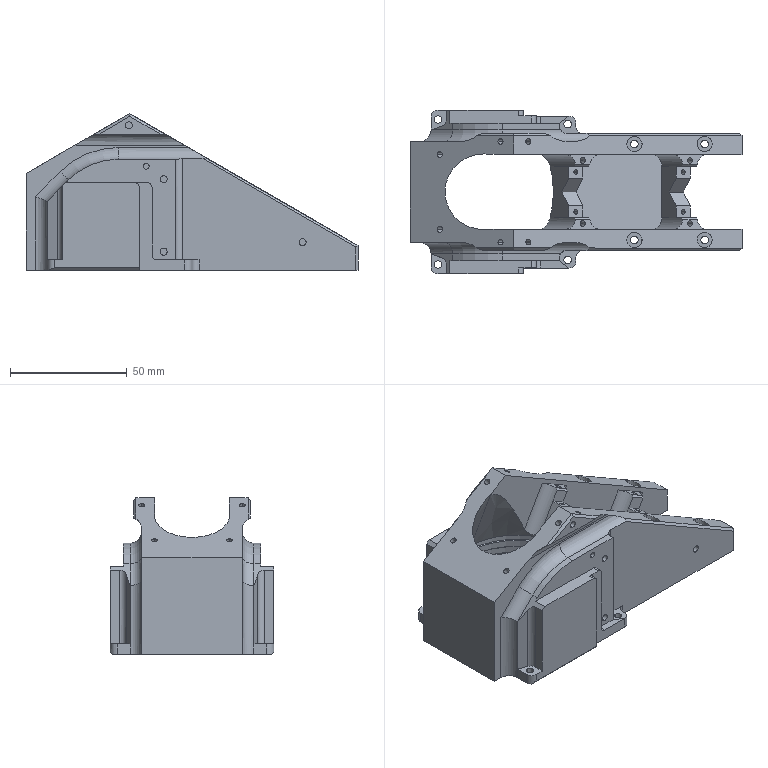CAM job | NX | 3-axis milling, drilling | part box 142 x 70 x 67 mm | stock box 142 x 70 x 67 mm
Tools:
number,name,description,diameter,corner_radius,flute_length,length,flutes
0,D80,Milling Tool-5 Parameters,80.0,0.0,50.0,75.0,2
0,DK-D12,Countersink,12.0,0.0,0.0,60.0,2
0,D05钻头,Drilling Tool,5.0,0.0,35.0,50.0,2
0,D4R0,Milling Tool-5 Parameters,4.0,0.0,50.0,75.0,2
0,D16R0波刀,Milling Tool-5 Parameters,16.0,0.0,50.0,75.0,2
0,D6R0,Milling Tool-5 Parameters,6.0,0.0,50.0,75.0,2
0,D10R0,Milling Tool-5 Parameters,10.0,0.0,40.0,40.0,2
0,DJ-D3,Countersink,3.0,0.0,0.0,60.0,2
0,DK-D5,Countersink,5.0,0.0,0.0,60.0,2
0,D6.5钻头,Drilling Tool,6.5,0.0,35.0,50.0,2
0,D3.2钻头,Drilling Tool,3.2,0.0,35.0,50.0,2
0,D6.5R0,Milling Tool-5 Parameters,6.5,0.0,50.0,75.0,2
0,M6,Drilling Tool,6.0,0.0,35.0,50.0,4
0,U钻-D21,Milling Tool-5 Parameters,21.0,1.0,30.0,30.0,4
17,D8R0,Milling Tool-5 Parameters,8.0,0.0,30.0,30.0,2
16,T10-1-T型刀,Milling Tool-T Cutter,10.0,,1.0,50.0,4
0,D18.5-0.5螺纹刀,Thread Mill,9.87,0.0,20.0,50.0,20
0,D2R0,Milling Tool-5 Parameters,2.0,0.0,50.0,75.0,2
0,D10.5,Drilling Tool,10.5,0.0,35.0,50.0,2
0,D2.5,Drilling Tool,2.5,0.0,35.0,50.0,2
0,M3,Drilling Tool,3.0,0.0,35.0,50.0,4
0,D50,Milling Tool-5 Parameters,50.0,0.0,50.0,75.0,2
15,D3R0,Milling Tool-5 Parameters,3.0,0.0,50.0,75.0,2
0,R5,Milling Tool-Ball Mill,10.0,5.0,50.0,75.0,2
0,D12R0,Milling Tool-5 Parameters,12.0,0.0,50.0,75.0,2
0,D12R0波刀,Milling Tool-5 Parameters,12.0,0.0,30.0,30.0,2
0,DK-D4,Countersink,4.0,0.0,0.0,60.0,2
18,D2.3钻头,Drilling Tool,2.3,0.0,35.0,50.0,2
0,D2.75钻头,Drilling Tool,2.75,0.0,35.0,50.0,2
0,D1.8钻头,Drilling Tool,1.8,0.0,35.0,50.0,2
0,M2.5,Drilling Tool,2.5,0.0,35.0,50.0,4
0,M2,Drilling Tool,2.0,0.0,35.0,50.0,4
0,D10R0精,Milling Tool-5 Parameters,9.95,0.0,55.0,55.0,2
Operations:
program,operation,operation_type,tool,method,geometry_group,spindle_rpm,surface_speed,feed_per_tooth,feed_cut,feed_plunge,cut_length_mm,path_length_mm,cut_time_min,machine_time_min
A01,FACE_MILLING,FaceMilling,D80,METHOD,WORKPIECE,2500.0,628.0,0.2,1000.0,100.0,246.0,311.4,0.246,0.2558
A01,DRILLING_COPY_2_COPY,Operation,U钻-D21,METHOD,A-G54,2000.0,131.0,0.0125,100.0,0.0,42.5,145.0,0.425,0.4352
A01,PLANAR_MILL_COPY,PlanarMilling,D16R0波刀,METHOD,A-G54,5500.0,276.0,0.2273,2500.0,100.0,10969.731,11458.321,4.388,4.44
A01,PLANAR_MILL_COPY_COPY_2,PlanarMilling,D16R0波刀,METHOD,A-G54,5500.0,276.0,0.1818,2000.0,100.0,1342.69,1481.29,0.6713,0.6885
A01,PLANAR_MILL_COPY_COPY_3,PlanarMilling,D16R0波刀,METHOD,A-G54,5500.0,276.0,0.2273,2500.0,100.0,707.2,956.428,0.2829,0.3111
A01,PLANAR_MILL_COPY_COPY_COPY_COPY_1,PlanarMilling,D10R0,METHOD,A-G54,3500.0,109.0,0.2571,1800.0,100.0,2232.499,4316.909,1.24,1.492
A01,PLANAR_MILL_COPY_COPY_COPY_COPY_1_COPY,PlanarMilling,D10R0,METHOD,A-G54,3500.0,109.0,0.2571,1800.0,100.0,3183.563,5741.476,1.769,2.068
A01,PLANAR_MILL_COPY_COPY_COPY_COPY_COPY_COPY_1,PlanarMilling,D10R0,METHOD,A-G54,2500.0,78.0,0.1,500.0,100.0,1221.661,3507.672,2.443,2.735
A01,PLANAR_MILL_COPY_COPY_COPY_COPY_COPY_COPY_1_COPY,PlanarMilling,D10R0,METHOD,A-G54,2500.0,78.0,0.1,500.0,100.0,872.574,2584.12,1.745,1.966
A01,PLANAR_MILL_COPY_COPY_COPY,PlanarMilling,D6R0,METHOD,A-G54,3000.0,56.0,0.2,1200.0,100.0,5065.863,9644.031,4.222,4.766
A01,PLANAR_MILL_COPY_COPY_COPY_COPY_2,PlanarMilling,D6R0,METHOD,A-G54,3000.0,56.0,0.0833,500.0,100.0,574.493,2289.263,1.149,1.384
A01,PLANAR_MILL_COPY_COPY_COPY_COPY_2_COPY_1,PlanarMilling,D6R0,METHOD,A-G54,3000.0,56.0,0.0833,500.0,100.0,699.355,2450.255,1.399,1.637
A01,PLANAR_MILL_COPY_COPY_COPY_COPY_2_COPY_1_COPY,PlanarMilling,D6R0,METHOD,A-G54,3000.0,56.0,0.0833,500.0,100.0,601.488,3079.829,1.203,1.553
A01,PLANAR_MILL_COPY_COPY_COPY_COPY_2_COPY,PlanarMilling,D6R0,METHOD,A-G54,3000.0,56.0,0.0833,500.0,100.0,64.809,996.356,0.1296,0.2598
A01,PLANAR_MILL_COPY_COPY_COPY_COPY_2_COPY_1_COPY_COPY,PlanarMilling,D6R0,METHOD,A-G54,3000.0,56.0,0.0833,500.0,100.0,954.479,4648.177,1.909,2.432
A01,DRILLING,Operation,DK-D12,METHOD,A-G54,1800.0,67.0,0.0556,200.0,0.0,18.0,350.764,0.09,0.1233
A01,DRILLING_COPY,Operation,DK-D12,METHOD,A-G54,1800.0,67.0,0.0556,200.0,0.0,10.8,188.921,0.054,0.0718
A01,DRILLING_COPY_2,Operation,DK-D12,METHOD,A-G54,1800.0,67.0,0.0556,200.0,0.0,22.0,281.729,0.11,0.136
A01,PLANAR_MILL_COPY_COPY_COPY_COPY_COPY_COPY,PlanarMilling,DK-D12,METHOD,A-G54,4000.0,150.0,0.125,1000.0,100.0,116.817,180.817,0.1168,0.1264
A01,PLANAR_MILL_COPY_COPY_COPY_COPY_COPY_COPY_COPY,PlanarMilling,DK-D12,METHOD,A-G54,4000.0,150.0,0.125,1000.0,100.0,59.85,123.85,0.0598,0.0694
A01,PLANAR_MILL_COPY_COPY_1_COPY_2,PlanarMilling,DK-D12,METHOD,A-G54,5500.0,51.0,0.0909,1000.0,100.0,431.064,493.364,0.4311,0.4404
A01,DRILLING_COPY_3,Operation,DK-D5,METHOD,A-G54,1500.0,23.0,0.0333,100.0,0.0,12.4,743.273,0.124,0.1971
A01,DRILLING_COPY_1,Operation,D05钻头,METHOD,A-G54,2000.0,31.0,0.05,200.0,0.0,74.0,462.764,0.37,0.4089
A01,DRILLING_COPY_1_COPY,Operation,D05钻头,METHOD,A-G54,2000.0,31.0,0.05,200.0,0.0,23.0,213.321,0.115,0.134
A01,DRILLING_COPY_1_COPY_1,Operation,D6.5钻头,METHOD,A-G54,2000.0,40.0,0.05,200.0,0.0,254.0,745.729,1.27,1.319
A01,DRILLING_COPY_1_COPY_1_COPY_1,Operation,D6.5R0,METHOD,A-G54,1200.0,24.0,0.0625,150.0,0.0,250.0,737.729,1.667,1.715
A01,HOLE_MILLING,CylinderMilling,D4R0,METHOD,A-G54,5500.0,69.0,0.1091,1200.0,100.0,456.402,677.802,0.3803,0.4084
A01,PLANAR_MILL,PlanarMilling,D4R0,METHOD,A-G54,5500.0,69.0,0.0364,400.0,100.0,65.781,302.796,0.1645,0.1958
A01,PLANAR_MILL_COPY_COPY_1,PlanarMilling,DJ-D3,METHOD,A-G54,5500.0,51.0,0.0909,1000.0,100.0,421.639,483.939,0.4216,0.431
A01,PLANAR_MILL_COPY_COPY_1_COPY_1,PlanarMilling,DJ-D3,METHOD,A-G54,5500.0,51.0,0.0909,1000.0,100.0,57.478,238.277,0.0575,0.0817
A01,PLANAR_MILL_COPY_COPY_1_COPY_1_COPY,PlanarMilling,DJ-D3,METHOD,A-G54,5500.0,51.0,0.0909,1000.0,100.0,35.076,210.793,0.0351,0.0588
A01,DRILLING_COPY_1_COPY_2,Operation,M6,METHOD,A-G54,300.0,5.0,0.0008,1.0,0.0,64.0,442.764,64.0,64.038
B01,FACE_MILLING_COPY,FaceMilling,D80,METHOD,B-G55,3500.0,879.0,0.2143,1500.0,100.0,984.0,1881.75,0.656,0.7538
B02,DRILLING_COPY_2_COPY_COPY,Operation,U钻-D21,METHOD,B-G55,2000.0,131.0,0.0125,100.0,0.0,36.5,133.0,0.365,0.3746
B03,CAVITY_MILL,CavityMilling,D16R0波刀,METHOD,B-G55,5500.0,276.0,0.2273,2500.0,100.0,4256.988,4647.488,1.703,1.748
B03,FIXED_CONTOUR,SurfaceContour,D16R0波刀,METHOD,B-G55,5500.0,276.0,0.2727,3000.0,100.0,4549.099,4686.463,1.516,1.536
B03,ZLEVEL_PROFILE,ZLevelMilling,D16R0波刀,METHOD,B-G55,5500.0,276.0,0.2727,3000.0,100.0,1925.687,2348.7,0.6419,0.6995
B04,FLOOR_WALL,VolumeBased25DMillingOperation,D8R0,METHOD,B-G55,5000.0,125.0,0.2,2000.0,100.0,2364.587,2554.954,1.182,1.206
B04,FLOOR_WALL_COPY,VolumeBased25DMillingOperation,D8R0,METHOD,B-G55,5000.0,125.0,0.06,600.0,100.0,119.366,196.366,0.1989,0.2105
B04,PLANAR_MILL_COPY_1_COPY,PlanarMilling,D8R0,METHOD,B-G55,5000.0,125.0,0.06,600.0,50.0,64.225,123.825,0.1432,0.1521
B04,PLANAR_MILL_COPY_1,PlanarMilling,D8R0,METHOD,B-G55,5000.0,125.0,0.06,600.0,100.0,93.825,170.825,0.1564,0.1679
B04,PLANAR_MILL_COPY_1_COPY_COPY,PlanarMilling,D8R0,METHOD,B-G55,5000.0,125.0,0.06,600.0,50.0,64.225,123.825,0.1432,0.1521
B05,PLANAR_MILL_COPY_COPY_COPY_COPY_COPY_2,PlanarMilling,D10R0,METHOD,B-G55,4500.0,141.0,0.1111,1000.0,100.0,464.0,1584.951,0.464,0.6147
B05,PLANAR_MILL_COPY_COPY_COPY_COPY_COPY_2_COPY_3,PlanarMilling,D10R0,METHOD,B-G55,4500.0,141.0,0.1111,1000.0,100.0,464.0,1584.951,0.464,0.6147
B05,PLANAR_MILL_COPY_COPY_COPY_COPY_COPY_2_COPY,PlanarMilling,D10R0,METHOD,B-G55,4500.0,141.0,0.1333,1200.0,100.0,558.407,630.407,0.4653,0.4761
B05,PLANAR_MILL_COPY_COPY_COPY_COPY_COPY_2_COPY_COPY,PlanarMilling,D10R0,METHOD,B-G55,4500.0,141.0,0.1333,1200.0,100.0,553.695,632.995,0.4614,0.4733
B05,PLANAR_MILL_COPY_COPY_COPY_COPY_COPY_2_COPY_COPY_COPY,PlanarMilling,D10R0,METHOD,B-G55,4500.0,141.0,0.1333,1200.0,100.0,534.845,599.145,0.4457,0.4553
B05,PLANAR_MILL_COPY_COPY_COPY_COPY_COPY_2_COPY_COPY_COPY_COPY,PlanarMilling,D10R0,METHOD,B-G55,4500.0,141.0,0.1333,1200.0,100.0,512.226,577.826,0.4269,0.4367
B05,PLANAR_MILL_COPY_COPY_COPY_COPY_COPY_2_COPY_COPY_COPY_COPY_COPY,PlanarMilling,D10R0,METHOD,B-G55,4500.0,141.0,0.1111,1000.0,100.0,501.858,570.958,0.5019,0.5122
B05,PLANAR_MILL_COPY_COPY_COPY_COPY_COPY_2_COPY_COPY_COPY_COPY_1,PlanarMilling,D10R0,METHOD,B-G55,4500.0,141.0,0.1111,1000.0,100.0,491.721,557.821,0.4917,0.5016
B06,DRILLING_COPY_3_COPY,Operation,DK-D5,METHOD,B-G55,1500.0,23.0,0.0333,100.0,0.0,24.8,576.563,0.248,0.3032
B06,DRILLING_COPY_3_COPY_COPY,Operation,DK-D5,METHOD,B-G55,1500.0,23.0,0.0333,100.0,0.0,6.2,138.018,0.062,0.0752
B06,PLANAR_MILL_COPY_COPY_1_COPY_COPY_COPY_1,PlanarMilling,DK-D5,METHOD,B-G55,5000.0,47.0,0.1,1000.0,100.0,421.199,483.199,0.4212,0.4305
B06,PLANAR_MILL_COPY_COPY_1_COPY_COPY_COPY_COPY_COPY_COPY,PlanarMilling,DK-D5,METHOD,B-G55,5000.0,47.0,0.04,400.0,100.0,198.699,515.302,0.4967,0.5358
B06,PLANAR_MILL_COPY_COPY_1_COPY_COPY_COPY_COPY_COPY_COPY_COPY,PlanarMilling,DK-D5,METHOD,B-G55,5000.0,47.0,0.04,400.0,100.0,198.699,515.302,0.4967,0.5358
B06,DRILLING_COPY_3_COPY_COPY_1,Operation,D3.2钻头,METHOD,B-G55,1500.0,23.0,0.0333,100.0,0.0,84.0,694.963,0.84,0.9011
B07,PLANAR_MILL_COPY_COPY_COPY_COPY_COPY_2_COPY_1_COPY_1,PlanarMilling,T10-1-T型刀,METHOD,B-G55,2000.0,62.0,0.0625,500.0,100.0,173.531,233.531,0.3471,0.3561
B08,PLANAR_MILL_COPY_COPY_1_COPY,PlanarMilling,DJ-D3,METHOD,B-G55,5000.0,47.0,0.1,1000.0,100.0,214.058,275.658,0.2141,0.2233
B08,PLANAR_MILL_COPY_COPY_1_COPY_COPY,PlanarMilling,DJ-D3,METHOD,B-G55,5000.0,47.0,0.1,1000.0,100.0,203.062,265.062,0.2031,0.2124
B08,PLANAR_MILL_COPY_COPY_1_COPY_COPY_COPY,PlanarMilling,DJ-D3,METHOD,B-G55,5000.0,47.0,0.1,1000.0,100.0,195.522,257.522,0.1955,0.2048
B08,PLANAR_MILL_COPY_COPY_1_COPY_COPY_COPY_COPY,PlanarMilling,DJ-D3,METHOD,B-G55,5000.0,47.0,0.1,1000.0,100.0,184.212,246.212,0.1842,0.1935
B08,PLANAR_MILL_COPY_COPY_1_COPY_COPY_1,PlanarMilling,DJ-D3,METHOD,B-G55,5000.0,47.0,0.1,1000.0,100.0,118.673,180.273,0.1187,0.1279
B08,PLANAR_MILL_COPY_COPY_1_COPY_COPY_1_COPY,PlanarMilling,DJ-D3,METHOD,B-G55,5000.0,47.0,0.1,1000.0,100.0,36.966,115.566,0.037,0.0488
B09,PLANAR_MILL_COPY_COPY_COPY_COPY_COPY_2_COPY_COPY_1,PlanarMilling,D10R0,METHOD,B-G55,4500.0,141.0,0.0889,800.0,100.0,183.783,255.783,0.2297,0.2405
B09,PLANAR_MILL_COPY_COPY_COPY_COPY_COPY_2_COPY_COPY_COPY_COPY_COPY_2,PlanarMilling,D10R0,METHOD,B-G55,4500.0,141.0,0.0889,800.0,100.0,168.389,233.989,0.2105,0.2203
B09,PLANAR_MILL_COPY_COPY_COPY_COPY_COPY_2_COPY_COPY_COPY_COPY_COPY_COPY,PlanarMilling,D10R0,METHOD,B-G55,4500.0,141.0,0.0889,800.0,100.0,164.934,234.034,0.2062,0.2165
B09,PLANAR_MILL_COPY_COPY_COPY_COPY_COPY_2_COPY_COPY_COPY_1,PlanarMilling,D10R0,METHOD,B-G55,4500.0,141.0,0.0667,600.0,100.0,378.376,457.776,0.6306,0.6425
B09,PLANAR_MILL_COPY_COPY_COPY_COPY_COPY_2_COPY_COPY_COPY_COPY_2,PlanarMilling,D10R0,METHOD,B-G55,4500.0,141.0,0.0667,600.0,100.0,365.81,430.21,0.6097,0.6193
B09,PLANAR_MILL_COPY_COPY_COPY_COPY_COPY_2_COPY_COPY_COPY_COPY_1_COPY,PlanarMilling,D10R0,METHOD,B-G55,4500.0,141.0,0.0667,600.0,100.0,161.096,227.296,0.2685,0.2784
B10,THREAD_MILLING,ThreadMilling,D18.5-0.5螺纹刀,METHOD,B-G55,4000.0,232.0,0.25,1000.0,100.0,1158.116,1239.73,1.158,1.17
B10,THREAD_MILLING_COPY,ThreadMilling,D18.5-0.5螺纹刀,METHOD,B-G55,4000.0,232.0,0.25,1000.0,100.0,1009.035,1089.992,1.009,1.021
B11,HOLE_MILLING_1,CylinderMilling,D2R0,METHOD,B-G55,6000.0,37.0,0.0417,500.0,100.0,69.424,236.054,0.1388,0.1615
B11,PLANAR_MILL_1,PlanarMilling,D2R0,METHOD,B-G55,6000.0,37.0,0.0167,200.0,100.0,23.481,196.711,0.1174,0.1413
B12,PLANAR_MILL_6,PlanarMilling,D4R0,METHOD,B-G55,4500.0,56.0,0.1111,1000.0,100.0,470.493,1718.781,0.4705,0.5953
B12,PLANAR_MILL_6_COPY,PlanarMilling,D4R0,METHOD,B-G55,4500.0,56.0,0.0444,400.0,100.0,95.604,355.797,0.239,0.265
B13,FACE_MILLING_COPY_COPY,FaceMilling,D80,METHOD,B-G55,3500.0,879.0,0.0857,600.0,100.0,246.0,322.0,0.41,0.4214
PROGRAM_1,PLANAR_PROFILE,PlanarMilling,D50,METHOD,C-G56,4500.0,706.0,0.2778,2500.0,100.0,2625.0,2726.7,1.05,1.063
PROGRAM_1,FACE_MILLING_1,FaceMilling,D50,METHOD,C-G56,4500.0,706.0,0.3333,3000.0,100.0,20987.492,22908.885,6.996,7.191
PROGRAM_1,FACE_MILLING_1_COPY,FaceMilling,D50,METHOD,C-G56,4500.0,706.0,0.3333,3000.0,100.0,10782.933,12226.109,3.594,3.74
PROGRAM_1,FACE_MILLING_1_COPY_1,FaceMilling,D50,METHOD,C-G56,4500.0,706.0,0.1111,1000.0,100.0,368.202,488.002,0.3682,0.3862
PROGRAM_1,FACE_MILLING_1_COPY_COPY,FaceMilling,D50,METHOD,C-G56,4500.0,706.0,0.1111,1000.0,100.0,245.067,304.867,0.2451,0.254
PROGRAM_1,FLOOR_WALL_2,VolumeBased25DMillingOperation,D12R0波刀,METHOD,C-G56,6000.0,226.0,0.2083,2500.0,100.0,7545.875,8157.103,3.018,3.084
PROGRAM_1,PLANAR_MILL_3_COPY_2,PlanarMilling,D12R0波刀,METHOD,C-G56,6000.0,226.0,0.1667,2000.0,100.0,3760.813,4802.007,1.88,1.988
PROGRAM_1,PLANAR_MILL_3_COPY_2_COPY,PlanarMilling,D12R0波刀,METHOD,C-G56,6000.0,226.0,0.2083,2500.0,100.0,4527.89,5524.939,1.811,1.914
PROGRAM_1,CAVITY_MILL_2_COPY_COPY_2_COPY,CavityMilling,D12R0波刀,METHOD,C-G56,6000.0,226.0,0.25,3000.0,100.0,1050.336,1285.637,0.3501,0.3828
PROGRAM_1,CAVITY_MILL_2_COPY_COPY_2,CavityMilling,D12R0波刀,METHOD,C-G56,6000.0,226.0,0.25,3000.0,100.0,135.825,313.825,0.0453,0.0693
PROGRAM_1,PLANAR_MILL_3_COPY_2_COPY_1,PlanarMilling,D12R0波刀,METHOD,C-G56,6000.0,226.0,0.25,3000.0,100.0,723.2,3651.6,0.2411,0.621
PROGRAM_1,CAVITY_MILL_2_COPY,CavityMilling,D12R0波刀,METHOD,C-G56,6000.0,226.0,0.375,4500.0,100.0,6288.489,6790.01,1.397,1.459
PROGRAM_1,CAVITY_MILL_2_COPY_COPY,CavityMilling,D12R0波刀,METHOD,C-G56,6000.0,226.0,0.375,4500.0,100.0,6171.071,6684.696,1.371,1.434
C01,ADAPTIVE_MILLING,CavityMilling,D12R0波刀,METHOD,WORKPIECE_1,6000.0,226.0,0.2083,2500.0,100.0,12501.855,12815.653,4.996,5.027
C01,ADAPTIVE_MILLING_COPY,CavityMilling,D12R0波刀,METHOD,WORKPIECE_1,6000.0,226.0,0.2083,2500.0,100.0,4381.51,4552.97,1.554,1.571
C01,PLANAR_MILL_3_COPY_2_COPY_3,PlanarMilling,D12R0波刀,METHOD,C-G56,6000.0,226.0,0.1667,2000.0,100.0,3760.813,4802.007,1.88,1.988
C01,ADAPTIVE_MILLING_COPY_1,CavityMilling,D12R0波刀,METHOD,WORKPIECE_1,6000.0,226.0,0.2083,2500.0,100.0,4466.184,4564.125,1.782,1.792
C01,PLANAR_MILL_3_COPY_2_COPY_COPY_1,PlanarMilling,D12R0波刀,METHOD,C-G56,6000.0,226.0,0.2083,2500.0,100.0,4527.89,5524.939,1.811,1.914
C01,CAVITY_MILL_2_COPY_COPY_2_COPY_COPY,CavityMilling,D12R0波刀,METHOD,C-G56,6000.0,226.0,0.25,3000.0,100.0,1050.336,1285.637,0.3501,0.3828
C01,CAVITY_MILL_2_COPY_COPY_2_COPY_1,CavityMilling,D12R0波刀,METHOD,C-G56,6000.0,226.0,0.25,3000.0,100.0,135.825,313.825,0.0453,0.0693
C01,PLANAR_MILL_3_COPY_2_COPY_1_COPY_1,PlanarMilling,D12R0波刀,METHOD,C-G56,6000.0,226.0,0.25,3000.0,100.0,723.2,3651.6,0.2411,0.621
C01,CAVITY_MILL_2_COPY_COPY_COPY_1,CavityMilling,D12R0波刀,METHOD,C-G56,6000.0,226.0,0.375,4500.0,100.0,6170.253,6683.877,1.371,1.434
C01,CAVITY_MILL_2_COPY_COPY_3,CavityMilling,D12R0波刀,METHOD,C-G56,6000.0,226.0,0.375,4500.0,100.0,6285.136,6788.874,1.397,1.458
C01,PLANAR_MILL_3_COPY_2_COPY_2_COPY,PlanarMilling,D8R0,METHOD,C-G56,6000.0,150.0,0.05,600.0,100.0,260.819,340.819,0.4347,0.4467
C01,FLOOR_WALL_2_COPY,VolumeBased25DMillingOperation,D8R0,METHOD,C-G56,6000.0,150.0,0.05,600.0,100.0,456.956,557.456,0.7616,0.7766
C01,PLANAR_MILL_3_COPY_2_COPY_2,PlanarMilling,D8R0,METHOD,C-G56,6000.0,150.0,0.05,600.0,100.0,361.669,486.226,0.6028,0.6195
C01,PLANAR_MILL_3_COPY_2_COPY_2_COPY_COPY,PlanarMilling,D8R0,METHOD,C-G56,6000.0,150.0,0.05,600.0,100.0,109.133,433.133,0.1819,0.2271
C01,PLANAR_MILL_3_COPY_2_COPY_COPY,PlanarMilling,D8R0,METHOD,C-G56,6000.0,150.0,0.0417,500.0,100.0,374.294,536.253,0.7486,0.7685
C01,PLANAR_MILL_3_COPY_2_COPY_2_COPY_COPY_COPY,PlanarMilling,D8R0,METHOD,C-G56,6000.0,150.0,0.05,600.0,100.0,69.6,420.4,0.116,0.1654
C01,PLANAR_MILL_3_COPY_2_COPY_1_COPY,PlanarMilling,D8R0,METHOD,C-G56,6000.0,150.0,0.05,600.0,100.0,69.6,384.046,0.116,0.1596
C01,PLANAR_MILL_3_COPY_2_COPY_1_COPY_COPY,PlanarMilling,D8R0,METHOD,C-G56,6000.0,150.0,0.05,600.0,100.0,34.8,190.4,0.058,0.0796
C01,PLANAR_MILL_7,PlanarMilling,D8R0,METHOD,C-G56,6500.0,163.0,0.0615,800.0,100.0,57.4,113.4,0.0718,0.0774
C01,PLANAR_MILL_7_COPY_1,PlanarMilling,D8R0,METHOD,C-G56,6500.0,163.0,0.0615,800.0,100.0,57.4,113.4,0.0718,0.0774
C01,PLANAR_MILL_7_COPY,PlanarMilling,D8R0,METHOD,C-G56,6500.0,163.0,0.0615,800.0,100.0,57.4,113.4,0.0717,0.0774
C01,PLANAR_MILL_7_COPY_COPY,PlanarMilling,D8R0,METHOD,C-G56,6500.0,163.0,0.0615,800.0,100.0,57.4,113.4,0.0717,0.0774
C01,FLOOR_FACING_1,VolumeBased25DMillingOperation,D8R0,METHOD,C-G56,6500.0,163.0,0.0615,800.0,100.0,80.603,143.675,0.1008,0.1071
C01,FLOOR_FACING_1_COPY_2,VolumeBased25DMillingOperation,D8R0,METHOD,C-G56,6500.0,163.0,0.0615,800.0,100.0,79.636,142.707,0.0995,0.1059
C01,FLOOR_FACING_1_COPY,VolumeBased25DMillingOperation,D8R0,METHOD,C-G56,6500.0,163.0,0.0615,800.0,100.0,37.578,102.77,0.047,0.0535
C01,FLOOR_FACING_1_COPY_COPY,VolumeBased25DMillingOperation,D8R0,METHOD,C-G56,6500.0,163.0,0.0615,800.0,100.0,37.129,102.321,0.0464,0.0529
C01,FLOOR_FACING_1_COPY_1,VolumeBased25DMillingOperation,D8R0,METHOD,C-G56,6500.0,163.0,0.0615,800.0,100.0,67.082,130.153,0.0839,0.0902
C01,FLOOR_FACING_1_COPY_1_COPY_1,VolumeBased25DMillingOperation,D8R0,METHOD,C-G56,6500.0,163.0,0.0615,800.0,100.0,66.282,129.353,0.0829,0.0892
C01,FLOOR_FACING_1_COPY_1_COPY,VolumeBased25DMillingOperation,D8R0,METHOD,C-G56,6500.0,163.0,0.0615,800.0,100.0,36.23,101.422,0.0453,0.0518
C01,FLOOR_FACING_1_COPY_1_COPY_COPY,VolumeBased25DMillingOperation,D8R0,METHOD,C-G56,6500.0,163.0,0.0615,800.0,100.0,35.806,100.998,0.0448,0.0513
C01,PLANAR_MILL_8,PlanarMilling,D8R0,METHOD,C-G56,6500.0,163.0,0.0615,800.0,100.0,18.749,74.749,0.0234,0.029
C01,PLANAR_MILL_8_COPY_1,PlanarMilling,D8R0,METHOD,C-G56,6500.0,163.0,0.0615,800.0,100.0,18.812,74.812,0.0235,0.0291
C01,PLANAR_MILL_8_COPY,PlanarMilling,D8R0,METHOD,C-G56,6500.0,163.0,0.0615,800.0,100.0,18.749,74.749,0.0234,0.029
C01,PLANAR_MILL_8_COPY_COPY,PlanarMilling,D8R0,METHOD,C-G56,6500.0,163.0,0.0615,800.0,100.0,18.812,74.812,0.0235,0.0291
C01,CAVITY_MILL_2_COPY_COPY_COPY,CavityMilling,D3R0,METHOD,C-G56,6500.0,61.0,0.2692,3500.0,100.0,1392.758,1671.649,0.3979,0.4347
C01,FLOOR_FACING_2,VolumeBased25DMillingOperation,D3R0,METHOD,C-G56,6500.0,61.0,0.0462,600.0,100.0,343.207,510.322,0.572,0.5887
C01,FLOOR_FACING_2_COPY_2,VolumeBased25DMillingOperation,D3R0,METHOD,C-G56,6500.0,61.0,0.0462,600.0,100.0,858.959,1417.65,1.432,1.488
C01,CAVITY_MILL_2_COPY_COPY_1,CavityMilling,D3R0,METHOD,C-G56,6500.0,61.0,0.2692,3500.0,100.0,1456.227,1874.6,0.4161,0.4706
C01,FLOOR_FACING_2_COPY,VolumeBased25DMillingOperation,D3R0,METHOD,C-G56,6500.0,61.0,0.0462,600.0,100.0,343.207,510.322,0.572,0.5887
C01,FLOOR_FACING_2_COPY_1,VolumeBased25DMillingOperation,D3R0,METHOD,C-G56,6500.0,61.0,0.0462,600.0,100.0,858.962,1417.653,1.432,1.488
C01,CAVITY_MILL_2,CavityMilling,D3R0,METHOD,C-G56,6500.0,61.0,0.0769,1000.0,100.0,219.463,284.463,0.2195,0.2292
C01,CAVITY_MILL_2_COPY_1,CavityMilling,D3R0,METHOD,C-G56,6500.0,61.0,0.0769,1000.0,100.0,450.058,521.258,0.4501,0.4607
C01,CAVITY_MILL_2_COPY_2,CavityMilling,D3R0,METHOD,C-G56,6500.0,61.0,0.0769,1000.0,100.0,219.463,284.463,0.2195,0.2292
C01,CAVITY_MILL_2_COPY_1_COPY_1,CavityMilling,D3R0,METHOD,C-G56,6500.0,61.0,0.0769,1000.0,100.0,450.058,521.258,0.4501,0.4607
C01,CAVITY_MILL_2_COPY_3,CavityMilling,D3R0,METHOD,C-G56,6500.0,61.0,0.0615,800.0,100.0,219.512,284.512,0.2744,0.2841
C01,FLOOR_FACING_2_COPY_COPY,VolumeBased25DMillingOperation,D3R0,METHOD,C-G56,6500.0,61.0,0.0462,600.0,100.0,171.625,254.625,0.286,0.2943
C01,FLOOR_FACING_2_COPY_1_COPY,VolumeBased25DMillingOperation,D3R0,METHOD,C-G56,6500.0,61.0,0.0462,600.0,100.0,113.283,194.383,0.1888,0.1969
C01,PLANAR_MILL_9_COPY,PlanarMilling,D3R0,METHOD,C-G56,6500.0,61.0,0.0462,600.0,100.0,43.445,106.445,0.0724,0.0787
C01,PLANAR_MILL_9_COPY_COPY,PlanarMilling,D3R0,METHOD,C-G56,6500.0,61.0,0.0462,600.0,100.0,68.957,124.957,0.1149,0.1205
C01,CAVITY_MILL_2_COPY_1_COPY_2,CavityMilling,D3R0,METHOD,C-G56,6500.0,61.0,0.0615,800.0,100.0,451.046,522.246,0.5638,0.5745
C01,CAVITY_MILL_2_COPY_2_COPY,CavityMilling,D3R0,METHOD,C-G56,6500.0,61.0,0.0615,800.0,100.0,219.512,284.512,0.2744,0.2841
C01,CAVITY_MILL_2_COPY_1_COPY_1_COPY,CavityMilling,D3R0,METHOD,C-G56,6500.0,61.0,0.0615,800.0,100.0,451.046,522.246,0.5638,0.5745
C01,FLOOR_FACING_2_COPY_3,VolumeBased25DMillingOperation,D3R0,METHOD,C-G56,6500.0,61.0,0.0462,600.0,100.0,171.625,254.625,0.286,0.2943
C01,FLOOR_FACING_2_COPY_2_COPY,VolumeBased25DMillingOperation,D3R0,METHOD,C-G56,6500.0,61.0,0.0462,600.0,100.0,107.605,188.705,0.1793,0.1875
C01,PLANAR_MILL_9_COPY_1,PlanarMilling,D3R0,METHOD,C-G56,6500.0,61.0,0.0462,600.0,100.0,68.957,124.957,0.1149,0.1205
C01,PLANAR_MILL_9,PlanarMilling,D3R0,METHOD,C-G56,6500.0,61.0,0.0462,600.0,100.0,43.445,106.445,0.0724,0.0787
C01,PLANAR_MILL_3,PlanarMilling,R5,METHOD,C-G56,5000.0,157.0,0.05,500.0,100.0,117.189,177.189,0.2344,0.2434
C01,PLANAR_MILL_3_COPY_3,PlanarMilling,R5,METHOD,C-G56,5000.0,157.0,0.05,500.0,100.0,117.189,177.189,0.2344,0.2434
C01,FIXED_CONTOUR_2,SurfaceContour,R5,METHOD,C-G56,5000.0,157.0,0.25,2500.0,100.0,990.323,1042.373,0.3961,0.4038
C01,PLANAR_MILL_3_COPY_1,PlanarMilling,R5,METHOD,C-G56,5000.0,157.0,0.05,500.0,100.0,120.16,180.161,0.2403,0.2493
C01,PLANAR_MILL_3_COPY_1_COPY,PlanarMilling,R5,METHOD,C-G56,5000.0,157.0,0.05,500.0,100.0,120.16,180.161,0.2403,0.2493
C01,FIXED_CONTOUR_2_COPY,SurfaceContour,R5,METHOD,C-G56,5000.0,157.0,0.25,2500.0,100.0,990.323,1042.373,0.3961,0.4038
C01,DRILLING_1,Operation,DK-D4,METHOD,C-G56,2000.0,37.0,0.05,200.0,0.0,11.0,263.632,0.055,0.0803
C01,DRILLING_1_COPY,Operation,DK-D4,METHOD,C-G56,2000.0,37.0,0.05,200.0,0.0,5.5,138.424,0.0275,0.0408
C01,DRILLING_1_COPY_COPY,Operation,DK-D4,METHOD,C-G56,2000.0,37.0,0.05,200.0,0.0,6.0,134.942,0.03,0.0429
C01,DRILLING_1_COPY_COPY_COPY,Operation,DK-D4,METHOD,C-G56,2000.0,37.0,0.05,200.0,0.0,11.0,288.897,0.055,0.0828
C01,DRILLING_1_COPY_COPY_COPY_COPY,Operation,DK-D4,METHOD,C-G56,2000.0,37.0,0.05,200.0,0.0,10.0,291.345,0.05,0.0781
C01,DRILLING_1_COPY_COPY_COPY_COPY_COPY,Operation,DK-D4,METHOD,C-G56,2000.0,37.0,0.05,200.0,0.0,12.0,276.766,0.06,0.0865
C01,DRILLING_1_COPY_COPY_COPY_COPY_COPY_COPY,Operation,DK-D4,METHOD,C-G56,2000.0,37.0,0.05,200.0,0.0,2.75,56.7,0.0138,0.0191
C01,DRILLING_1_COPY_COPY_COPY_COPY_COPY_COPY_1,Operation,DK-D4,METHOD,C-G56,2000.0,37.0,0.05,200.0,0.0,12.0,313.748,0.06,0.0902
C01,DRILLING_1_COPY_COPY_COPY_COPY_COPY_COPY_COPY,Operation,DK-D4,METHOD,C-G56,2000.0,37.0,0.05,200.0,0.0,2.75,65.5,0.0138,0.02
C01,PLANAR_MILL_4_COPY_COPY_COPY_COPY,PlanarMilling,DK-D4,METHOD,C-G56,4000.0,37.0,0.1,800.0,100.0,307.053,528.659,0.3838,0.4102
C01,PLANAR_MILL_4_COPY_COPY_COPY_COPY_COPY,PlanarMilling,DK-D4,METHOD,C-G56,4000.0,37.0,0.1,800.0,100.0,307.053,528.659,0.3838,0.4102
C01,DRILLING_1_COPY_1,Operation,D2.3钻头,METHOD,C-G56,2000.0,14.0,0.0375,150.0,0.0,16.4,150.536,0.1093,0.1227
C01,DRILLING_1_COPY_1_COPY_2,Operation,D2.3钻头,METHOD,C-G56,2000.0,14.0,0.0375,150.0,0.0,12.0,151.424,0.08,0.0939
C01,DRILLING_1_COPY_1_COPY,Operation,D2.3钻头,METHOD,C-G56,2000.0,14.0,0.0375,150.0,0.0,12.0,151.424,0.08,0.0939
C01,DRILLING_1_COPY_1_COPY_COPY,Operation,D2.3钻头,METHOD,C-G56,2000.0,14.0,0.0375,150.0,0.0,38.0,342.897,0.2533,0.2838
C01,DRILLING_1_COPY_1_COPY_COPY_COPY,Operation,D2.3钻头,METHOD,C-G56,2000.0,14.0,0.0375,150.0,0.0,9.0,78.0,0.06,0.0669
C01,DRILLING_1_COPY_1_COPY_COPY_COPY_COPY,Operation,D2.3钻头,METHOD,C-G56,2000.0,14.0,0.0375,150.0,0.0,9.0,69.2,0.06,0.066
C01,DRILLING_1_COPY_COPY_COPY_1,Operation,D2.75钻头,METHOD,C-G56,2000.0,37.0,0.05,200.0,0.0,18.0,158.942,0.09,0.1041
C01,DRILLING_1_COPY_COPY_COPY_1_COPY,Operation,D2.75钻头,METHOD,C-G56,2000.0,37.0,0.05,200.0,0.0,19.0,209.763,0.095,0.1141
C01,DRILLING_1_COPY_COPY_COPY_1_COPY_COPY,Operation,D2.75钻头,METHOD,C-G56,2000.0,37.0,0.05,200.0,0.0,14.0,136.092,0.07,0.0822
C01,DRILLING_1_COPY_COPY_COPY_1_COPY_COPY_1,Operation,D2.75钻头,METHOD,C-G56,2000.0,37.0,0.05,200.0,0.0,19.0,209.763,0.095,0.1141
C01,DRILLING_1_COPY_COPY_COPY_1_COPY_COPY_COPY,Operation,D2.75钻头,METHOD,C-G56,2000.0,37.0,0.05,200.0,0.0,14.0,144.892,0.07,0.0831
C01,DRILLING_1_COPY_COPY_COPY_COPY_COPY_1,Operation,D1.8钻头,METHOD,C-G56,2000.0,25.0,0.025,100.0,0.0,34.0,339.345,0.34,0.3705
C01,DRILLING_1_COPY_1_COPY_2_COPY,Operation,D2.3钻头,METHOD,C-G56,2000.0,14.0,0.0375,150.0,0.0,12.0,151.424,0.08,0.0939
C01,DRILLING_1_COPY_1_COPY_COPY_2,Operation,D2.3钻头,METHOD,C-G56,2000.0,14.0,0.0375,150.0,0.0,12.0,151.424,0.08,0.0939
C01,PLANAR_MILL_4,PlanarMilling,DJ-D3,METHOD,C-G56,4000.0,37.0,0.125,1000.0,100.0,112.176,173.776,0.1122,0.1214
C01,PLANAR_MILL_4_COPY,PlanarMilling,DJ-D3,METHOD,C-G56,4000.0,37.0,0.125,1000.0,100.0,53.829,120.829,0.0538,0.0639
C01,PLANAR_MILL_4_COPY_COPY,PlanarMilling,DJ-D3,METHOD,C-G56,4000.0,37.0,0.125,1000.0,100.0,93.892,167.092,0.0939,0.1049
C01,PLANAR_MILL_4_COPY_COPY_COPY,PlanarMilling,DJ-D3,METHOD,C-G56,4000.0,37.0,0.125,1000.0,100.0,28.445,90.445,0.0284,0.0377
C01,PLANAR_MILL_4_COPY_2,PlanarMilling,DJ-D3,METHOD,C-G56,4000.0,37.0,0.125,1000.0,100.0,112.176,173.776,0.1122,0.1214
C01,PLANAR_MILL_4_COPY_COPY_1,PlanarMilling,DJ-D3,METHOD,C-G56,4000.0,37.0,0.125,1000.0,100.0,53.829,120.829,0.0538,0.0639
C01,PLANAR_MILL_4_COPY_COPY_COPY_1,PlanarMilling,DJ-D3,METHOD,C-G56,4000.0,37.0,0.125,1000.0,100.0,93.892,167.092,0.0939,0.1049
C01,PLANAR_MILL_4_COPY_COPY_COPY_COPY_1,PlanarMilling,DJ-D3,METHOD,C-G56,4000.0,37.0,0.125,1000.0,100.0,28.445,90.445,0.0284,0.0377
C01,PLANAR_MILL_4_COPY_1,PlanarMilling,DJ-D3,METHOD,C-G56,4000.0,37.0,0.125,1000.0,100.0,79.341,248.359,0.0793,0.1024
C01,PLANAR_MILL_4_COPY_1_COPY_COPY,PlanarMilling,DJ-D3,METHOD,C-G56,4000.0,37.0,0.1,800.0,100.0,92.541,154.541,0.1157,0.125
C01,PLANAR_MILL_4_COPY_1_COPY_COPY_COPY,PlanarMilling,DJ-D3,METHOD,C-G56,4000.0,37.0,0.125,1000.0,100.0,235.935,389.517,0.2359,0.2575
C01,PLANAR_MILL_4_COPY_1_COPY_COPY_COPY_COPY,PlanarMilling,DJ-D3,METHOD,C-G56,4000.0,37.0,0.125,1000.0,100.0,32.233,186.215,0.0322,0.0538
C01,VARIABLE_CONTOUR,SurfaceContour,D10R0精,METHOD,C-G56,3500.0,109.0,0.0429,300.0,100.0,493.903,598.525,1.646,1.658
C01,VARIABLE_CONTOUR_COPY_COPY,SurfaceContour,D10R0精,METHOD,C-G56,3000.0,94.0,0.05,300.0,100.0,740.857,860.686,2.47,2.483
C01,DRILLING_1_COPY_1_COPY_1,Operation,M2.5,METHOD,C-G56,400.0,2.0,0.225,180.0,0.0,15.0,147.736,0.0833,0.0966
C01,DRILLING_1_COPY_1_COPY_1_COPY,Operation,M2.5,METHOD,C-G56,400.0,2.0,0.225,180.0,0.0,11.8,151.024,0.0656,0.0795
C01,DRILLING_1_COPY_1_COPY_COPY_1,Operation,M2.5,METHOD,C-G56,400.0,2.0,0.225,180.0,0.0,11.6,150.624,0.0644,0.0783
C01,DRILLING_1_COPY_1_COPY_COPY_COPY_1,Operation,M2.5,METHOD,C-G56,400.0,2.0,0.225,180.0,0.0,32.0,330.897,0.1778,0.2077
C01,DRILLING_1_COPY_1_COPY_COPY_COPY_COPY_1,Operation,M2.5,METHOD,C-G56,400.0,2.0,0.225,180.0,0.0,8.0,76.0,0.0444,0.0512
C01,DRILLING_1_COPY_1_COPY_COPY_COPY_COPY_COPY,Operation,M2.5,METHOD,C-G56,400.0,2.0,0.225,180.0,0.0,8.0,67.2,0.0444,0.0504
C01,DRILLING_1_COPY_COPY_COPY_1_COPY_1,Operation,M3,METHOD,C-G56,400.0,3.0,0.25,200.0,0.0,14.6,152.142,0.073,0.0868
C01,DRILLING_1_COPY_COPY_COPY_1_COPY_COPY_2,Operation,M3,METHOD,C-G56,400.0,3.0,0.25,200.0,0.0,17.0,205.763,0.085,0.1039
C01,DRILLING_1_COPY_COPY_COPY_1_COPY_COPY_COPY_1,Operation,M3,METHOD,C-G56,400.0,3.0,0.25,200.0,0.0,12.0,132.092,0.06,0.072
C01,DRILLING_1_COPY_COPY_COPY_1_COPY_COPY_1_COPY,Operation,M3,METHOD,C-G56,400.0,3.0,0.25,200.0,0.0,17.0,205.763,0.085,0.1039
C01,DRILLING_1_COPY_COPY_COPY_1_COPY_COPY_COPY_COPY,Operation,M3,METHOD,C-G56,400.0,3.0,0.25,200.0,0.0,12.0,140.892,0.06,0.0729
C01,DRILLING_1_COPY_COPY_COPY_COPY_COPY_1_COPY,Operation,M2,METHOD,C-G56,400.0,2.0,0.1,160.0,0.0,28.0,327.345,0.175,0.2049
C01,FLOOR_FACING_COPY_COPY,VolumeBased25DMillingOperation,D8R0,METHOD,C-G56,5500.0,138.0,0.0909,1000.0,100.0,294.851,354.851,0.2949,0.3009
C01,FACE_MILLING_2,FaceMilling,D8R0,METHOD,C-G56,6000.0,150.0,0.05,600.0,100.0,70.725,150.726,0.1179,0.1299
C01,FLOOR_FACING_COPY_COPY_1,VolumeBased25DMillingOperation,D8R0,METHOD,C-G56,5500.0,138.0,0.0909,1000.0,100.0,292.799,352.799,0.2928,0.2988
C01,FACE_MILLING_2_COPY,FaceMilling,D8R0,METHOD,C-G56,6000.0,150.0,0.05,600.0,100.0,70.725,150.726,0.1179,0.1299
C01,FLOOR_FACING,VolumeBased25DMillingOperation,D8R0,METHOD,C-G56,5500.0,138.0,0.0909,1000.0,100.0,512.502,675.094,0.5125,0.5288
C01,FLOOR_FACING_COPY,VolumeBased25DMillingOperation,D8R0,METHOD,C-G56,5500.0,138.0,0.0909,1000.0,100.0,407.058,467.058,0.4071,0.4131
C01,FLOOR_FACING_COPY_COPY_2,VolumeBased25DMillingOperation,D8R0,METHOD,C-G56,5500.0,138.0,0.0909,1000.0,100.0,405.219,465.219,0.4052,0.4112
C01,FLOOR_FACING_COPY_COPY_2_COPY,VolumeBased25DMillingOperation,D8R0,METHOD,C-G56,5500.0,138.0,0.0909,1000.0,100.0,104.064,266.863,0.1041,0.1203
三轴工装,CAVITY_MILL_1,CavityMilling,D16R0波刀,METHOD,工装1,5000.0,251.0,0.2,2000.0,100.0,4814.914,4931.914,2.408,2.423
三轴工装,DRILLING_COPY_2_COPY_COPY_1,Operation,U钻-D21,METHOD,工装1,2000.0,131.0,0.0125,100.0,0.0,32.5,125.0,0.325,0.3342
三轴工装,DRILLING_COPY_4,Operation,DK-D12,METHOD,工装1,1800.0,67.0,0.0556,200.0,0.0,18.0,350.764,0.09,0.1233
三轴工装,DRILLING_COPY_1_COPY_1_COPY_2,Operation,D6.5钻头,METHOD,工装1,2000.0,40.0,0.05,200.0,0.0,146.0,606.764,0.73,0.7761
三轴工装,CAVITY_MILL_1_COPY,CavityMilling,D4R0,METHOD,工装1,6000.0,75.0,0.1667,2000.0,100.0,6519.965,6585.965,3.26,3.27
三轴工装,PLANAR_TEXT,Engraving,DJ-D3,METHOD,工装1,5000.0,47.0,0.06,600.0,100.0,241.325,1100.357,0.4022,0.5208
三轴工装,PLANAR_MILL_2_COPY,PlanarMilling,DJ-D3,METHOD,工装1,5000.0,47.0,0.1,1000.0,100.0,73.685,281.579,0.0737,0.1006
三轴工装,PLANAR_MILL_2_COPY_COPY,PlanarMilling,DJ-D3,METHOD,工装1,5000.0,47.0,0.1,1000.0,100.0,80.197,141.596,0.0802,0.0894
三轴工装,PLANAR_MILL_2_COPY_COPY_COPY,PlanarMilling,DJ-D3,METHOD,工装1,5000.0,47.0,0.1,1000.0,100.0,531.71,593.11,0.5317,0.5409
PROGRAM,PLANAR_MILL_2,PlanarMilling,D4R0,METHOD,工装1,5000.0,62.0,0.05,500.0,100.0,89.016,305.71,0.2315,0.2597
五轴工装,PLANAR_MILL_2_COPY_COPY_1,PlanarMilling,D16R0波刀,METHOD,工装2,5000.0,47.0,0.1,1000.0,100.0,3885.617,4108.993,3.886,3.911
五轴工装,CAVITY_MILL_1_COPY_1,CavityMilling,D16R0波刀,METHOD,工装2,5000.0,251.0,0.2,2000.0,100.0,2891.535,2992.685,1.446,1.459
五轴工装,CAVITY_MILL_1_COPY_1_COPY,CavityMilling,D16R0波刀,METHOD,工装2,5000.0,251.0,0.2,2000.0,100.0,1170.568,1290.098,0.5853,0.6009
五轴工装,DRILLING_COPY_4_COPY,Operation,DK-D12,METHOD,工装2,1800.0,67.0,0.0556,200.0,0.0,9.0,208.02,0.045,0.0649
五轴工装,DRILLING_COPY_4_COPY_COPY_1,Operation,DK-D12,METHOD,工装2,1800.0,67.0,0.0556,200.0,0.0,18.0,485.422,0.09,0.1367
五轴工装,DRILLING_COPY_4_COPY_COPY_COPY,Operation,D2.5,METHOD,工装2,1500.0,49.0,0.05,150.0,0.0,117.0,677.422,0.78,0.836
五轴工装,DRILLING_COPY_4_COPY_COPY,Operation,D10.5,METHOD,工装2,1500.0,49.0,0.05,150.0,0.0,97.0,378.02,0.6467,0.6748
五轴工装,DRILLING_COPY_4_COPY_COPY_COPY_COPY,Operation,M3,METHOD,工装2,400.0,3.0,0.125,200.0,0.0,39.0,521.422,0.195,0.2432
五轴工装,PLANAR_MILL_2_COPY_COPY_1_COPY,PlanarMilling,D10R0,METHOD,工装2,5000.0,47.0,0.1,1000.0,100.0,437.867,526.667,0.4379,0.4498
五轴工装,PLANAR_MILL_2_COPY_COPY_1_COPY_COPY,PlanarMilling,D10R0,METHOD,工装2,5000.0,47.0,0.1,1000.0,100.0,875.735,995.534,0.8757,0.8908
五轴工装,PLANAR_MILL_2_COPY_COPY_1_COPY_1,PlanarMilling,D10R0,METHOD,工装2,4000.0,125.0,0.1,800.0,100.0,1347.309,1458.733,1.684,1.699
五轴工装,PLANAR_MILL_2_COPY_COPY_1_COPY_1_COPY,PlanarMilling,DK-D12,METHOD,工装2,4000.0,150.0,0.125,1000.0,100.0,428.663,492.462,0.4287,0.4382
五轴工装,PLANAR_MILL_2_COPY_COPY_1_COPY_1_COPY_COPY,PlanarMilling,DK-D12,METHOD,工装2,4000.0,150.0,0.125,1000.0,100.0,150.483,216.283,0.1505,0.1604
1.H,CAVITY_MILL_3_COPY,CavityMilling,D12R0,METHOD,3,5500.0,207.0,0.1364,1500.0,100.0,6952.636,7378.888,4.635,4.686
1.H,CAVITY_MILL_3_COPY_COPY_1,CavityMilling,D12R0,METHOD,3,5000.0,471.0,0.04,400.0,100.0,200.417,294.83,0.501,0.5152
1.H,CAVITY_MILL_3,CavityMilling,D12R0,METHOD,3,4000.0,100.0,0.1,800.0,100.0,1459.482,1758.784,1.824,1.864
1.H,PLANAR_MILL_5,PlanarMilling,D12R0,METHOD,3,4000.0,100.0,0.05,400.0,100.0,239.57,395.725,0.5989,0.6191
2.H,PLANAR_MILL_5_COPY,PlanarMilling,D12R0,METHOD,3,4000.0,100.0,0.05,400.0,100.0,282.044,354.024,0.7051,0.7159
五轴工装精,PLANAR_MILL_5_COPY_1,PlanarMilling,DK-D5,METHOD,3,4000.0,37.0,0.125,1000.0,100.0,44.782,180.182,0.0448,0.0626